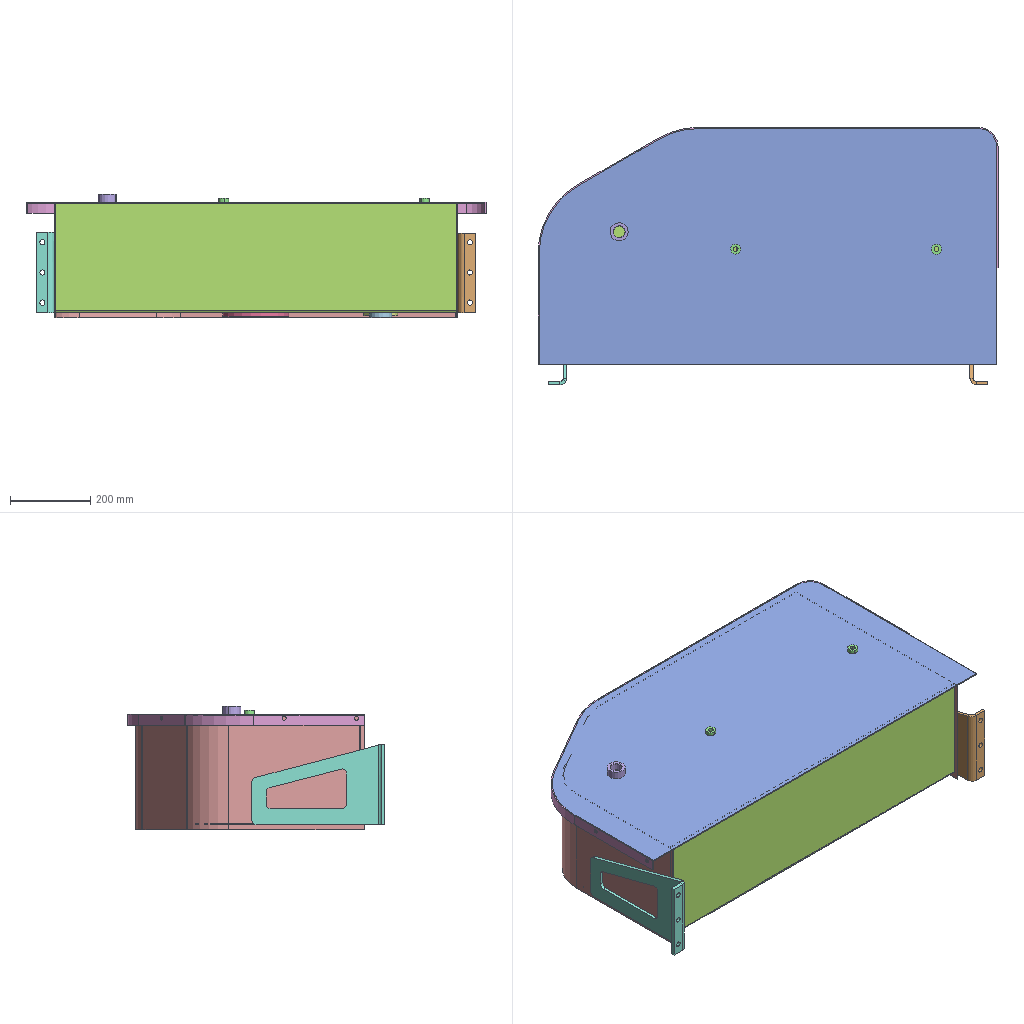Assembly | SolidWorks | 11 different items | 12 placed | box 1145 x 640 x 308 mm
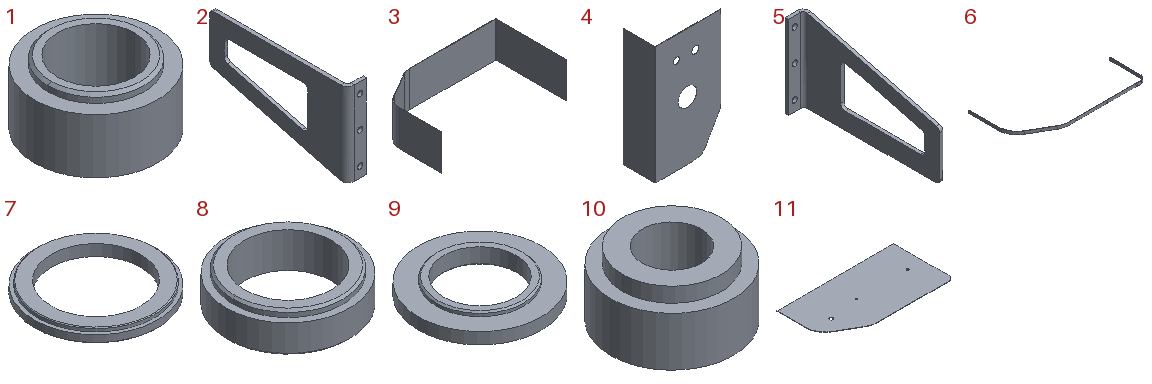Parts list (item | quantity | size | volume | features):
1 | x1 | 45 x 45 x 23 mm | 20434 mm3 | features 3DProfileFeature 1, Chamfer 1, Extrusion 1, HoleWzd 1, ICE 1
2 | x1 | 45 x 330 x 200 mm | 345586 mm3 | features ICE 2, FlatPattern 1, SMBaseFlange 1, SheetMetal 1
3 | x1 | 1004 x 570 x 285 mm | 1713041 mm3 | features FlatPattern 1, SMBaseFlange 1, SheetMetal 1
4 | x1 | 557 x 272 x 999 mm | 2327658 mm3 | features FlatPattern 1, ICE 1, SMBaseFlange 1, SheetMetal 1
5 | x1 | 45 x 330 x 197.939 mm | 342210 mm3 | features ICE 2, FlatPattern 1, SMBaseFlange 1, SheetMetal 1
6 | x1 | 1145 x 590 x 28 mm | 157323 mm3 | features Cut 2, FlatPattern 1, ICE 1, SMBaseFlange 1, SheetMetal 1
7 | x1 | 165 x 165 x 15 mm | 136481 mm3 | features 3DProfileFeature 1, Chamfer 1, Extrusion 1, HoleWzd 1, ICE 1
8 | x1 | 56 x 56 x 16 mm | 18386 mm3 | features 3DProfileFeature 1, Chamfer 1, Extrusion 1, HoleWzd 1, ICE 1
9 | x1 | 85 x 85 x 11 mm | 31782 mm3 | features 3DProfileFeature 1, Chamfer 1, Extrusion 1, HoleWzd 1, ICE 1
10 | x2 | 25 x 25 x 13 mm | 4381 mm3 | features 3DProfileFeature 1, Extrusion 1, HoleWzd 1, ICE 1
11 | x1 | 1139 x 587 x 3 mm | 1890389 mm3 | features Extrusion 1
Mates (type | each side: item.copy, entity, surface, feature):
Coincident | 11.1 face plane Boss-Extrude1 | 6.1 face plane Base-Flange1 | 3 times
DistanceDim | 3.1 face plane Base-Flange1 | 11.1 face plane Boss-Extrude1
DistanceDim | 4.1 face plane Base-Flange1 | 11.1 face plane Boss-Extrude1
Coincident | 3.1 face plane Base-Flange1 | 11.1 face plane Boss-Extrude1
Coincident | 11.1 face plane Boss-Extrude1 | 4.1 face plane Base-Flange1
Coincident | 3.1 face plane Base-Flange1 | 4.1 face plane Base-Flange1 | 2 times
Coincident | 3.1 face plane Base-Flange1 | 5.1 face plane Base-Flange1
DistanceDim | 5.1 face plane Base-Flange1 | 3.1 face plane Base-Flange1
Coincident | 4.1 face plane Base-Flange1 | 5.1 face plane Base-Flange1
Coincident | 2.1 face plane Base-Flange1 | 5.1 face plane Base-Flange1 | 2 times
Coincident | 3.1 face plane Base-Flange1 | 2.1 face plane Base-Flange1
Concentric | 11.1 edge | 1.1 edge
Coincident | 11.1 face plane Boss-Extrude1 | 1.1 face plane Boss-Extrude1
Concentric | 11.1 edge | 10.1 edge
Coincident | 11.1 face plane Boss-Extrude1 | 10.1 face plane Boss-Extrude1
Concentric | 11.1 edge | 10.2 edge
Coincident | 11.1 face plane Boss-Extrude1 | 10.2 face plane Boss-Extrude1
Concentric | 4.1 edge | 7.1 edge
Coincident | 4.1 face plane Base-Flange1 | 7.1 face plane Boss-Extrude1
Concentric | 4.1 edge | 8.1 edge
Coincident | 4.1 face plane Base-Flange1 | 8.1 face plane Boss-Extrude1
Concentric | 4.1 edge | 9.1 edge
Coincident | 4.1 face plane Base-Flange1 | 9.1 face plane Boss-Extrude1